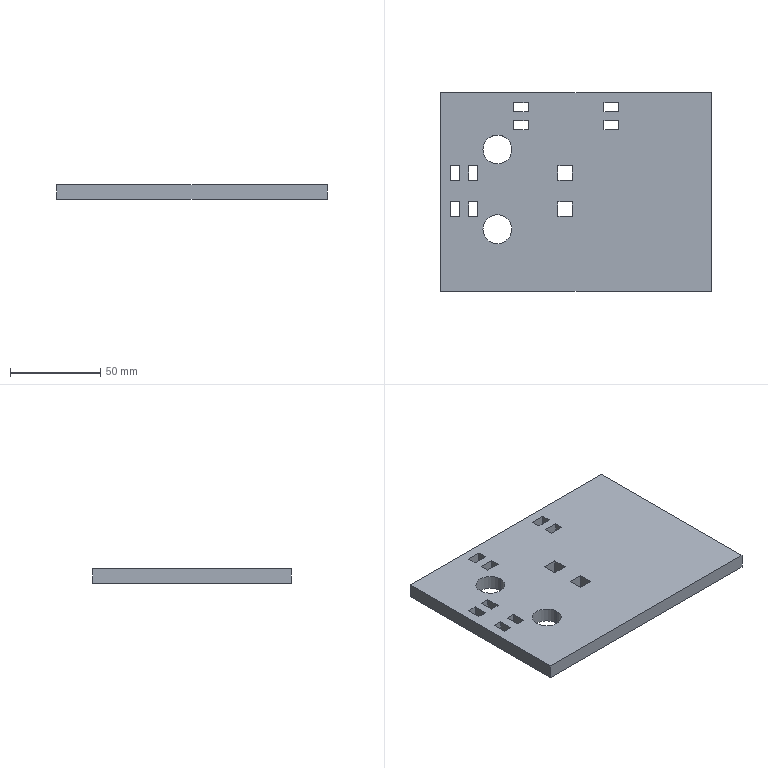Part | SolidWorks | features FlatPattern 1, SMBaseFlange 1, SheetMetal 1 | 1 solid | 50 faces | box 150 x 110 x 8 mm | volume 125199 mm3 | plane 46 | cylinder 4 | commonest cylinder face diameters 16 x4